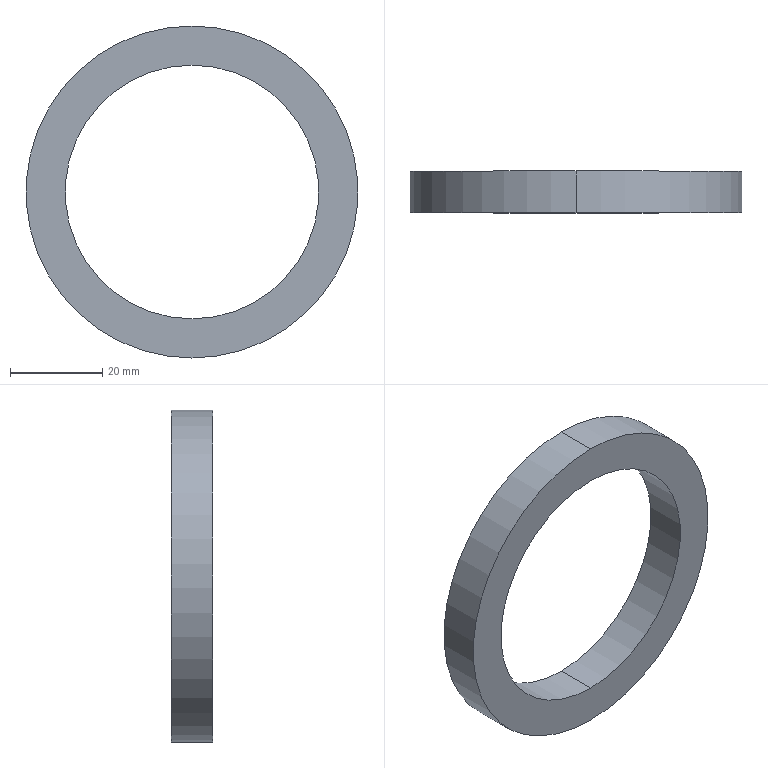Part | SolidWorks | features BaseBody 1 | 1 solid | 6 faces | box 72 x 9 x 72 mm | volume 15261 mm3 | cylinder 4 | plane 2 | commonest cylinder face diameters 55 x2 72 x2
STEP:
#1=CARTESIAN_POINT('',(0.,9.,27.5));
#2=VERTEX_POINT('',#1);
#3=CARTESIAN_POINT('',(0.,9.,-27.5));
#4=VERTEX_POINT('',#3);
#5=CARTESIAN_POINT('',(0.,9.,0.));
#6=DIRECTION('',(0.,-1.,0.));
#7=DIRECTION('',(0.,0.,-1.));
#8=AXIS2_PLACEMENT_3D('',#5,#6,#7);
#9=CIRCLE('',#8,27.5);
#10=EDGE_CURVE('',#2,#4,#9,.T.);
#11=ORIENTED_EDGE('',*,*,#10,.F.);
#12=CARTESIAN_POINT('',(0.,0.,27.5));
#13=VERTEX_POINT('',#12);
#14=CARTESIAN_POINT('',(0.,9.,27.5));
#15=DIRECTION('',(0.,-1.,0.));
#16=VECTOR('',#15,1000.);
#17=LINE('',#14,#16);
#18=EDGE_CURVE('',#2,#13,#17,.T.);
#19=ORIENTED_EDGE('',*,*,#18,.T.);
#20=CARTESIAN_POINT('',(0.,0.,-27.5));
#21=VERTEX_POINT('',#20);
#22=CARTESIAN_POINT('',(0.,0.,0.));
#23=DIRECTION('',(0.,1.,0.));
#24=DIRECTION('',(0.,0.,-1.));
#25=AXIS2_PLACEMENT_3D('',#22,#23,#24);
#26=CIRCLE('',#25,27.5);
#27=EDGE_CURVE('',#21,#13,#26,.T.);
#28=ORIENTED_EDGE('',*,*,#27,.F.);
#29=CARTESIAN_POINT('',(0.,9.,-27.5));
#30=DIRECTION('',(0.,-1.,0.));
#31=VECTOR('',#30,1000.);
#32=LINE('',#29,#31);
#33=EDGE_CURVE('',#4,#21,#32,.T.);
#34=ORIENTED_EDGE('',*,*,#33,.F.);
#35=EDGE_LOOP('',(#11,#19,#28,#34));
#36=FACE_OUTER_BOUND('',#35,.T.);
#37=CARTESIAN_POINT('',(0.,9.,0.));
#38=DIRECTION('',(0.,-1.,0.));
#39=DIRECTION('',(0.,0.,-1.));
#40=AXIS2_PLACEMENT_3D('',#37,#38,#39);
#41=CYLINDRICAL_SURFACE('',#40,27.5);
#42=ADVANCED_FACE('',(#36),#41,.F.);
#43=CARTESIAN_POINT('',(0.,9.,36.));
#44=VERTEX_POINT('',#43);
#45=CARTESIAN_POINT('',(0.,9.,-36.));
#46=VERTEX_POINT('',#45);
#47=CARTESIAN_POINT('',(0.,9.,0.));
#48=DIRECTION('',(0.,1.,0.));
#49=DIRECTION('',(0.,0.,-1.));
#50=AXIS2_PLACEMENT_3D('',#47,#48,#49);
#51=CIRCLE('',#50,36.);
#52=EDGE_CURVE('',#44,#46,#51,.T.);
#53=ORIENTED_EDGE('',*,*,#52,.F.);
#54=CARTESIAN_POINT('',(0.,0.,36.));
#55=VERTEX_POINT('',#54);
#56=CARTESIAN_POINT('',(0.,9.,36.));
#57=DIRECTION('',(0.,-1.,0.));
#58=VECTOR('',#57,1000.);
#59=LINE('',#56,#58);
#60=EDGE_CURVE('',#44,#55,#59,.T.);
#61=ORIENTED_EDGE('',*,*,#60,.T.);
#62=CARTESIAN_POINT('',(0.,0.,-36.));
#63=VERTEX_POINT('',#62);
#64=CARTESIAN_POINT('',(0.,0.,0.));
#65=DIRECTION('',(0.,1.,0.));
#66=DIRECTION('',(0.,0.,-1.));
#67=AXIS2_PLACEMENT_3D('',#64,#65,#66);
#68=CIRCLE('',#67,36.);
#69=EDGE_CURVE('',#55,#63,#68,.T.);
#70=ORIENTED_EDGE('',*,*,#69,.T.);
#71=CARTESIAN_POINT('',(0.,9.,-36.));
#72=DIRECTION('',(0.,-1.,0.));
#73=VECTOR('',#72,1000.);
#74=LINE('',#71,#73);
#75=EDGE_CURVE('',#46,#63,#74,.T.);
#76=ORIENTED_EDGE('',*,*,#75,.F.);
#77=EDGE_LOOP('',(#53,#61,#70,#76));
#78=FACE_OUTER_BOUND('',#77,.T.);
#79=CARTESIAN_POINT('',(0.,9.,0.));
#80=DIRECTION('',(0.,-1.,0.));
#81=DIRECTION('',(0.,0.,-1.));
#82=AXIS2_PLACEMENT_3D('',#79,#80,#81);
#83=CYLINDRICAL_SURFACE('',#82,36.);
#84=ADVANCED_FACE('',(#78),#83,.T.);
#85=CARTESIAN_POINT('',(0.,9.,0.));
#86=DIRECTION('',(0.,-1.,0.));
#87=DIRECTION('',(0.,0.,-1.));
#88=AXIS2_PLACEMENT_3D('',#85,#86,#87);
#89=CIRCLE('',#88,27.5);
#90=EDGE_CURVE('',#4,#2,#89,.T.);
#91=ORIENTED_EDGE('',*,*,#90,.T.);
#92=ORIENTED_EDGE('',*,*,#10,.T.);
#93=EDGE_LOOP('',(#91,#92));
#94=FACE_BOUND('',#93,.T.);
#95=CARTESIAN_POINT('',(0.,9.,0.));
#96=DIRECTION('',(0.,1.,0.));
#97=DIRECTION('',(0.,0.,-1.));
#98=AXIS2_PLACEMENT_3D('',#95,#96,#97);
#99=CIRCLE('',#98,36.);
#100=EDGE_CURVE('',#46,#44,#99,.T.);
#101=ORIENTED_EDGE('',*,*,#100,.T.);
#102=ORIENTED_EDGE('',*,*,#52,.T.);
#103=EDGE_LOOP('',(#101,#102));
#104=FACE_OUTER_BOUND('',#103,.T.);
#105=CARTESIAN_POINT('',(0.,9.,0.));
#106=DIRECTION('',(0.,1.,0.));
#107=DIRECTION('',(0.,0.,1.));
#108=AXIS2_PLACEMENT_3D('',#105,#106,#107);
#109=PLANE('',#108);
#110=ADVANCED_FACE('',(#94,#104),#109,.T.);
#111=ORIENTED_EDGE('',*,*,#18,.F.);
#112=ORIENTED_EDGE('',*,*,#90,.F.);
#113=ORIENTED_EDGE('',*,*,#33,.T.);
#114=CARTESIAN_POINT('',(0.,0.,0.));
#115=DIRECTION('',(0.,1.,0.));
#116=DIRECTION('',(0.,0.,-1.));
#117=AXIS2_PLACEMENT_3D('',#114,#115,#116);
#118=CIRCLE('',#117,27.5);
#119=EDGE_CURVE('',#13,#21,#118,.T.);
#120=ORIENTED_EDGE('',*,*,#119,.F.);
#121=EDGE_LOOP('',(#111,#112,#113,#120));
#122=FACE_OUTER_BOUND('',#121,.T.);
#123=CARTESIAN_POINT('',(0.,9.,0.));
#124=DIRECTION('',(0.,-1.,0.));
#125=DIRECTION('',(0.,0.,-1.));
#126=AXIS2_PLACEMENT_3D('',#123,#124,#125);
#127=CYLINDRICAL_SURFACE('',#126,27.5);
#128=ADVANCED_FACE('',(#122),#127,.F.);
#129=ORIENTED_EDGE('',*,*,#60,.F.);
#130=ORIENTED_EDGE('',*,*,#100,.F.);
#131=ORIENTED_EDGE('',*,*,#75,.T.);
#132=CARTESIAN_POINT('',(0.,0.,0.));
#133=DIRECTION('',(0.,1.,0.));
#134=DIRECTION('',(0.,0.,-1.));
#135=AXIS2_PLACEMENT_3D('',#132,#133,#134);
#136=CIRCLE('',#135,36.);
#137=EDGE_CURVE('',#63,#55,#136,.T.);
#138=ORIENTED_EDGE('',*,*,#137,.T.);
#139=EDGE_LOOP('',(#129,#130,#131,#138));
#140=FACE_OUTER_BOUND('',#139,.T.);
#141=CARTESIAN_POINT('',(0.,9.,0.));
#142=DIRECTION('',(0.,-1.,0.));
#143=DIRECTION('',(0.,0.,-1.));
#144=AXIS2_PLACEMENT_3D('',#141,#142,#143);
#145=CYLINDRICAL_SURFACE('',#144,36.);
#146=ADVANCED_FACE('',(#140),#145,.T.);
#147=ORIENTED_EDGE('',*,*,#27,.T.);
#148=ORIENTED_EDGE('',*,*,#119,.T.);
#149=EDGE_LOOP('',(#147,#148));
#150=FACE_BOUND('',#149,.T.);
#151=ORIENTED_EDGE('',*,*,#137,.F.);
#152=ORIENTED_EDGE('',*,*,#69,.F.);
#153=EDGE_LOOP('',(#151,#152));
#154=FACE_OUTER_BOUND('',#153,.T.);
#155=CARTESIAN_POINT('',(0.,0.,0.));
#156=DIRECTION('',(0.,1.,0.));
#157=DIRECTION('',(0.,0.,1.));
#158=AXIS2_PLACEMENT_3D('',#155,#156,#157);
#159=PLANE('',#158);
#160=ADVANCED_FACE('',(#150,#154),#159,.F.);
#161=CLOSED_SHELL('',(#42,#84,#110,#128,#146,#160));
#162=MANIFOLD_SOLID_BREP('',#161);
#163=CARTESIAN_POINT('',(0.,0.,0.));
#164=DIRECTION('',(0.,0.,1.));
#165=DIRECTION('',(1.,0.,0.));
#166=AXIS2_PLACEMENT_3D('',#163,#164,#165);
#167=(LENGTH_UNIT()NAMED_UNIT(*)SI_UNIT(.MILLI.,.METRE.));
#168=UNCERTAINTY_MEASURE_WITH_UNIT(LENGTH_MEASURE(0.00001),#167,'','');
#169=(NAMED_UNIT(*)PLANE_ANGLE_UNIT()SI_UNIT($,.RADIAN.));
#170=(NAMED_UNIT(*)SI_UNIT($,.STERADIAN.)SOLID_ANGLE_UNIT());
#171=(GEOMETRIC_REPRESENTATION_CONTEXT(3)GLOBAL_UNCERTAINTY_ASSIGNED_CONTEXT((#168))GLOBAL_UNIT_ASSIGNED_CONTEXT((#167,#169,#170))REPRESENTATION_CONTEXT('',''));
#172=ADVANCED_BREP_SHAPE_REPRESENTATION('',(#162,#166),#171);